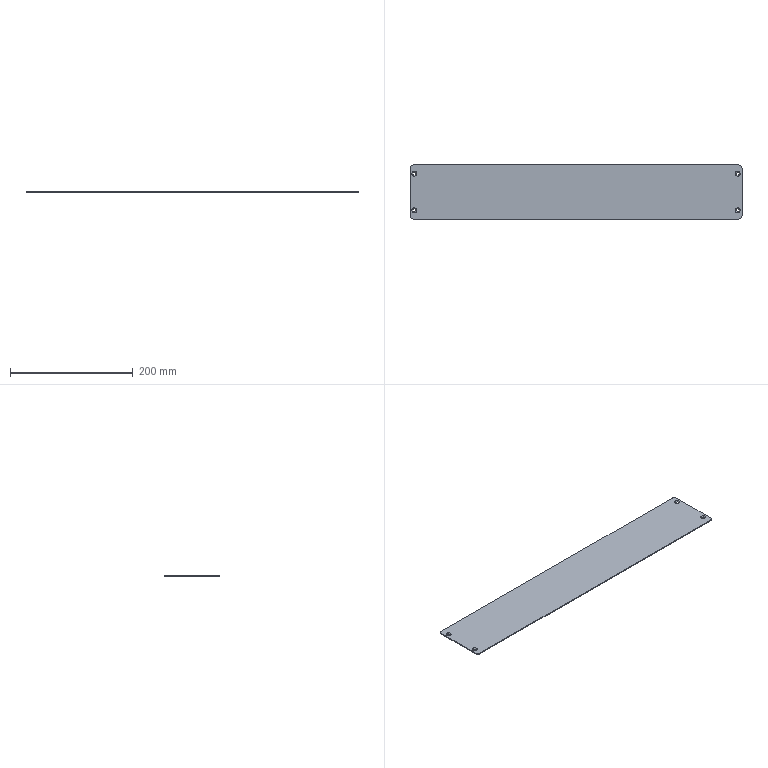Part | SolidWorks | features BreakCorner 1, Chamfer 1, FlatPattern 1, ICE 1, SMBaseFlange 1, SheetMetal 1 | 1 solid | 18 faces | box 541 x 88 x 1.5 mm | volume 71177 mm3 | cone 8 | plane 6 | cylinder 4 | commonest cylinder face diameters 10 x4
STEP:
#1=CARTESIAN_POINT('',(-266.,30.,-1.5));
#2=VERTEX_POINT('',#1);
#3=CARTESIAN_POINT('',(-261.,30.,-1.5));
#4=VERTEX_POINT('',#3);
#5=CARTESIAN_POINT('',(-263.5,30.,-1.5));
#6=DIRECTION('',(0.,0.,1.));
#7=DIRECTION('',(1.,0.,0.));
#8=AXIS2_PLACEMENT_3D('',#5,#6,#7);
#9=CIRCLE('',#8,2.5);
#10=EDGE_CURVE('',#2,#4,#9,.T.);
#11=ORIENTED_EDGE('',*,*,#10,.F.);
#12=CARTESIAN_POINT('',(-267.5,30.,0.));
#13=VERTEX_POINT('',#12);
#14=CARTESIAN_POINT('',(-266.,30.,-1.5));
#15=DIRECTION('',(-0.7071,0.,0.7071));
#16=VECTOR('',#15,1000.);
#17=LINE('',#14,#16);
#18=EDGE_CURVE('',#2,#13,#17,.T.);
#19=ORIENTED_EDGE('',*,*,#18,.T.);
#20=CARTESIAN_POINT('',(-259.5,30.,0.));
#21=VERTEX_POINT('',#20);
#22=CARTESIAN_POINT('',(-263.5,30.,0.));
#23=DIRECTION('',(0.,0.,-1.));
#24=DIRECTION('',(1.,0.,0.));
#25=AXIS2_PLACEMENT_3D('',#22,#23,#24);
#26=CIRCLE('',#25,4.);
#27=EDGE_CURVE('',#21,#13,#26,.T.);
#28=ORIENTED_EDGE('',*,*,#27,.F.);
#29=CARTESIAN_POINT('',(-261.,30.,-1.5));
#30=DIRECTION('',(0.7071,0.,0.7071));
#31=VECTOR('',#30,1000.);
#32=LINE('',#29,#31);
#33=EDGE_CURVE('',#4,#21,#32,.T.);
#34=ORIENTED_EDGE('',*,*,#33,.F.);
#35=EDGE_LOOP('',(#11,#19,#28,#34));
#36=FACE_OUTER_BOUND('',#35,.T.);
#37=CARTESIAN_POINT('',(-263.5,30.,-1.5));
#38=DIRECTION('',(0.,0.,1.));
#39=DIRECTION('',(1.,0.,0.));
#40=AXIS2_PLACEMENT_3D('',#37,#38,#39);
#41=CONICAL_SURFACE('',#40,2.5,0.7854);
#42=ADVANCED_FACE('',(#36),#41,.F.);
#43=CARTESIAN_POINT('',(-266.,-30.,-1.5));
#44=VERTEX_POINT('',#43);
#45=CARTESIAN_POINT('',(-261.,-30.,-1.5));
#46=VERTEX_POINT('',#45);
#47=CARTESIAN_POINT('',(-263.5,-30.,-1.5));
#48=DIRECTION('',(0.,0.,1.));
#49=DIRECTION('',(1.,0.,0.));
#50=AXIS2_PLACEMENT_3D('',#47,#48,#49);
#51=CIRCLE('',#50,2.5);
#52=EDGE_CURVE('',#44,#46,#51,.T.);
#53=ORIENTED_EDGE('',*,*,#52,.F.);
#54=CARTESIAN_POINT('',(-267.5,-30.,0.));
#55=VERTEX_POINT('',#54);
#56=CARTESIAN_POINT('',(-266.,-30.,-1.5));
#57=DIRECTION('',(-0.7071,0.,0.7071));
#58=VECTOR('',#57,1000.);
#59=LINE('',#56,#58);
#60=EDGE_CURVE('',#44,#55,#59,.T.);
#61=ORIENTED_EDGE('',*,*,#60,.T.);
#62=CARTESIAN_POINT('',(-259.5,-30.,0.));
#63=VERTEX_POINT('',#62);
#64=CARTESIAN_POINT('',(-263.5,-30.,0.));
#65=DIRECTION('',(0.,0.,-1.));
#66=DIRECTION('',(1.,0.,0.));
#67=AXIS2_PLACEMENT_3D('',#64,#65,#66);
#68=CIRCLE('',#67,4.);
#69=EDGE_CURVE('',#63,#55,#68,.T.);
#70=ORIENTED_EDGE('',*,*,#69,.F.);
#71=CARTESIAN_POINT('',(-261.,-30.,-1.5));
#72=DIRECTION('',(0.7071,0.,0.7071));
#73=VECTOR('',#72,1000.);
#74=LINE('',#71,#73);
#75=EDGE_CURVE('',#46,#63,#74,.T.);
#76=ORIENTED_EDGE('',*,*,#75,.F.);
#77=EDGE_LOOP('',(#53,#61,#70,#76));
#78=FACE_OUTER_BOUND('',#77,.T.);
#79=CARTESIAN_POINT('',(-263.5,-30.,-1.5));
#80=DIRECTION('',(0.,0.,1.));
#81=DIRECTION('',(1.,0.,0.));
#82=AXIS2_PLACEMENT_3D('',#79,#80,#81);
#83=CONICAL_SURFACE('',#82,2.5,0.7854);
#84=ADVANCED_FACE('',(#78),#83,.F.);
#85=CARTESIAN_POINT('',(261.,30.,-1.5));
#86=VERTEX_POINT('',#85);
#87=CARTESIAN_POINT('',(266.,30.,-1.5));
#88=VERTEX_POINT('',#87);
#89=CARTESIAN_POINT('',(263.5,30.,-1.5));
#90=DIRECTION('',(0.,0.,1.));
#91=DIRECTION('',(1.,0.,0.));
#92=AXIS2_PLACEMENT_3D('',#89,#90,#91);
#93=CIRCLE('',#92,2.5);
#94=EDGE_CURVE('',#86,#88,#93,.T.);
#95=ORIENTED_EDGE('',*,*,#94,.F.);
#96=CARTESIAN_POINT('',(259.5,30.,0.));
#97=VERTEX_POINT('',#96);
#98=CARTESIAN_POINT('',(261.,30.,-1.5));
#99=DIRECTION('',(-0.7071,0.,0.7071));
#100=VECTOR('',#99,1000.);
#101=LINE('',#98,#100);
#102=EDGE_CURVE('',#86,#97,#101,.T.);
#103=ORIENTED_EDGE('',*,*,#102,.T.);
#104=CARTESIAN_POINT('',(267.5,30.,0.));
#105=VERTEX_POINT('',#104);
#106=CARTESIAN_POINT('',(263.5,30.,0.));
#107=DIRECTION('',(0.,0.,-1.));
#108=DIRECTION('',(1.,0.,0.));
#109=AXIS2_PLACEMENT_3D('',#106,#107,#108);
#110=CIRCLE('',#109,4.);
#111=EDGE_CURVE('',#105,#97,#110,.T.);
#112=ORIENTED_EDGE('',*,*,#111,.F.);
#113=CARTESIAN_POINT('',(266.,30.,-1.5));
#114=DIRECTION('',(0.7071,0.,0.7071));
#115=VECTOR('',#114,1000.);
#116=LINE('',#113,#115);
#117=EDGE_CURVE('',#88,#105,#116,.T.);
#118=ORIENTED_EDGE('',*,*,#117,.F.);
#119=EDGE_LOOP('',(#95,#103,#112,#118));
#120=FACE_OUTER_BOUND('',#119,.T.);
#121=CARTESIAN_POINT('',(263.5,30.,-1.5));
#122=DIRECTION('',(0.,0.,1.));
#123=DIRECTION('',(1.,0.,0.));
#124=AXIS2_PLACEMENT_3D('',#121,#122,#123);
#125=CONICAL_SURFACE('',#124,2.5,0.7854);
#126=ADVANCED_FACE('',(#120),#125,.F.);
#127=CARTESIAN_POINT('',(261.,-30.,-1.5));
#128=VERTEX_POINT('',#127);
#129=CARTESIAN_POINT('',(266.,-30.,-1.5));
#130=VERTEX_POINT('',#129);
#131=CARTESIAN_POINT('',(263.5,-30.,-1.5));
#132=DIRECTION('',(0.,0.,1.));
#133=DIRECTION('',(1.,0.,0.));
#134=AXIS2_PLACEMENT_3D('',#131,#132,#133);
#135=CIRCLE('',#134,2.5);
#136=EDGE_CURVE('',#128,#130,#135,.T.);
#137=ORIENTED_EDGE('',*,*,#136,.F.);
#138=CARTESIAN_POINT('',(259.5,-30.,0.));
#139=VERTEX_POINT('',#138);
#140=CARTESIAN_POINT('',(261.,-30.,-1.5));
#141=DIRECTION('',(-0.7071,0.,0.7071));
#142=VECTOR('',#141,1000.);
#143=LINE('',#140,#142);
#144=EDGE_CURVE('',#128,#139,#143,.T.);
#145=ORIENTED_EDGE('',*,*,#144,.T.);
#146=CARTESIAN_POINT('',(267.5,-30.,0.));
#147=VERTEX_POINT('',#146);
#148=CARTESIAN_POINT('',(263.5,-30.,0.));
#149=DIRECTION('',(0.,0.,-1.));
#150=DIRECTION('',(1.,0.,0.));
#151=AXIS2_PLACEMENT_3D('',#148,#149,#150);
#152=CIRCLE('',#151,4.);
#153=EDGE_CURVE('',#147,#139,#152,.T.);
#154=ORIENTED_EDGE('',*,*,#153,.F.);
#155=CARTESIAN_POINT('',(266.,-30.,-1.5));
#156=DIRECTION('',(0.7071,0.,0.7071));
#157=VECTOR('',#156,1000.);
#158=LINE('',#155,#157);
#159=EDGE_CURVE('',#130,#147,#158,.T.);
#160=ORIENTED_EDGE('',*,*,#159,.F.);
#161=EDGE_LOOP('',(#137,#145,#154,#160));
#162=FACE_OUTER_BOUND('',#161,.T.);
#163=CARTESIAN_POINT('',(263.5,-30.,-1.5));
#164=DIRECTION('',(0.,0.,1.));
#165=DIRECTION('',(1.,0.,0.));
#166=AXIS2_PLACEMENT_3D('',#163,#164,#165);
#167=CONICAL_SURFACE('',#166,2.5,0.7854);
#168=ADVANCED_FACE('',(#162),#167,.F.);
#169=CARTESIAN_POINT('',(270.5,-39.,-1.5));
#170=VERTEX_POINT('',#169);
#171=CARTESIAN_POINT('',(270.5,39.,-1.5));
#172=VERTEX_POINT('',#171);
#173=CARTESIAN_POINT('',(270.5,44.,-1.5));
#174=DIRECTION('',(0.,1.,0.));
#175=VECTOR('',#174,1000.);
#176=LINE('',#173,#175);
#177=EDGE_CURVE('',#170,#172,#176,.T.);
#178=ORIENTED_EDGE('',*,*,#177,.T.);
#179=CARTESIAN_POINT('',(270.5,39.,0.));
#180=VERTEX_POINT('',#179);
#181=CARTESIAN_POINT('',(270.5,39.,-1.5));
#182=DIRECTION('',(0.,0.,1.));
#183=VECTOR('',#182,1000.);
#184=LINE('',#181,#183);
#185=EDGE_CURVE('',#172,#180,#184,.T.);
#186=ORIENTED_EDGE('',*,*,#185,.T.);
#187=CARTESIAN_POINT('',(270.5,-39.,0.));
#188=VERTEX_POINT('',#187);
#189=CARTESIAN_POINT('',(270.5,44.,0.));
#190=DIRECTION('',(0.,1.,0.));
#191=VECTOR('',#190,1000.);
#192=LINE('',#189,#191);
#193=EDGE_CURVE('',#188,#180,#192,.T.);
#194=ORIENTED_EDGE('',*,*,#193,.F.);
#195=CARTESIAN_POINT('',(270.5,-39.,-1.5));
#196=DIRECTION('',(0.,0.,-1.));
#197=VECTOR('',#196,1000.);
#198=LINE('',#195,#197);
#199=EDGE_CURVE('',#188,#170,#198,.T.);
#200=ORIENTED_EDGE('',*,*,#199,.T.);
#201=EDGE_LOOP('',(#178,#186,#194,#200));
#202=FACE_OUTER_BOUND('',#201,.T.);
#203=CARTESIAN_POINT('',(270.5,44.,-1.5));
#204=DIRECTION('',(1.,0.,0.));
#205=DIRECTION('',(0.,0.,-1.));
#206=AXIS2_PLACEMENT_3D('',#203,#204,#205);
#207=PLANE('',#206);
#208=ADVANCED_FACE('',(#202),#207,.T.);
#209=CARTESIAN_POINT('',(-265.5,-44.,-1.5));
#210=VERTEX_POINT('',#209);
#211=CARTESIAN_POINT('',(265.5,-44.,-1.5));
#212=VERTEX_POINT('',#211);
#213=CARTESIAN_POINT('',(-270.5,-44.,-1.5));
#214=DIRECTION('',(1.,0.,0.));
#215=VECTOR('',#214,1000.);
#216=LINE('',#213,#215);
#217=EDGE_CURVE('',#210,#212,#216,.T.);
#218=ORIENTED_EDGE('',*,*,#217,.T.);
#219=CARTESIAN_POINT('',(265.5,-44.,0.));
#220=VERTEX_POINT('',#219);
#221=CARTESIAN_POINT('',(265.5,-44.,-1.5));
#222=DIRECTION('',(0.,0.,1.));
#223=VECTOR('',#222,1000.);
#224=LINE('',#221,#223);
#225=EDGE_CURVE('',#212,#220,#224,.T.);
#226=ORIENTED_EDGE('',*,*,#225,.T.);
#227=CARTESIAN_POINT('',(-265.5,-44.,0.));
#228=VERTEX_POINT('',#227);
#229=CARTESIAN_POINT('',(-270.5,-44.,0.));
#230=DIRECTION('',(1.,0.,0.));
#231=VECTOR('',#230,1000.);
#232=LINE('',#229,#231);
#233=EDGE_CURVE('',#228,#220,#232,.T.);
#234=ORIENTED_EDGE('',*,*,#233,.F.);
#235=CARTESIAN_POINT('',(-265.5,-44.,-1.5));
#236=DIRECTION('',(0.,0.,-1.));
#237=VECTOR('',#236,1000.);
#238=LINE('',#235,#237);
#239=EDGE_CURVE('',#228,#210,#238,.T.);
#240=ORIENTED_EDGE('',*,*,#239,.T.);
#241=EDGE_LOOP('',(#218,#226,#234,#240));
#242=FACE_OUTER_BOUND('',#241,.T.);
#243=CARTESIAN_POINT('',(-270.5,-44.,-1.5));
#244=DIRECTION('',(0.,-1.,0.));
#245=DIRECTION('',(0.,0.,-1.));
#246=AXIS2_PLACEMENT_3D('',#243,#244,#245);
#247=PLANE('',#246);
#248=ADVANCED_FACE('',(#242),#247,.T.);
#249=CARTESIAN_POINT('',(-270.5,39.,-1.5));
#250=VERTEX_POINT('',#249);
#251=CARTESIAN_POINT('',(-270.5,-39.,-1.5));
#252=VERTEX_POINT('',#251);
#253=CARTESIAN_POINT('',(-270.5,44.,-1.5));
#254=DIRECTION('',(0.,-1.,0.));
#255=VECTOR('',#254,1000.);
#256=LINE('',#253,#255);
#257=EDGE_CURVE('',#250,#252,#256,.T.);
#258=ORIENTED_EDGE('',*,*,#257,.T.);
#259=CARTESIAN_POINT('',(-270.5,-39.,0.));
#260=VERTEX_POINT('',#259);
#261=CARTESIAN_POINT('',(-270.5,-39.,-1.5));
#262=DIRECTION('',(0.,0.,1.));
#263=VECTOR('',#262,1000.);
#264=LINE('',#261,#263);
#265=EDGE_CURVE('',#252,#260,#264,.T.);
#266=ORIENTED_EDGE('',*,*,#265,.T.);
#267=CARTESIAN_POINT('',(-270.5,39.,0.));
#268=VERTEX_POINT('',#267);
#269=CARTESIAN_POINT('',(-270.5,44.,0.));
#270=DIRECTION('',(0.,-1.,0.));
#271=VECTOR('',#270,1000.);
#272=LINE('',#269,#271);
#273=EDGE_CURVE('',#268,#260,#272,.T.);
#274=ORIENTED_EDGE('',*,*,#273,.F.);
#275=CARTESIAN_POINT('',(-270.5,39.,-1.5));
#276=DIRECTION('',(0.,0.,-1.));
#277=VECTOR('',#276,1000.);
#278=LINE('',#275,#277);
#279=EDGE_CURVE('',#268,#250,#278,.T.);
#280=ORIENTED_EDGE('',*,*,#279,.T.);
#281=EDGE_LOOP('',(#258,#266,#274,#280));
#282=FACE_OUTER_BOUND('',#281,.T.);
#283=CARTESIAN_POINT('',(-270.5,44.,-1.5));
#284=DIRECTION('',(-1.,0.,0.));
#285=DIRECTION('',(0.,0.,1.));
#286=AXIS2_PLACEMENT_3D('',#283,#284,#285);
#287=PLANE('',#286);
#288=ADVANCED_FACE('',(#282),#287,.T.);
#289=CARTESIAN_POINT('',(265.5,44.,0.));
#290=VERTEX_POINT('',#289);
#291=CARTESIAN_POINT('',(-265.5,44.,0.));
#292=VERTEX_POINT('',#291);
#293=CARTESIAN_POINT('',(-270.5,44.,0.));
#294=DIRECTION('',(-1.,0.,0.));
#295=VECTOR('',#294,1000.);
#296=LINE('',#293,#295);
#297=EDGE_CURVE('',#290,#292,#296,.T.);
#298=ORIENTED_EDGE('',*,*,#297,.F.);
#299=CARTESIAN_POINT('',(265.5,44.,-1.5));
#300=VERTEX_POINT('',#299);
#301=CARTESIAN_POINT('',(265.5,44.,-1.5));
#302=DIRECTION('',(0.,0.,-1.));
#303=VECTOR('',#302,1000.);
#304=LINE('',#301,#303);
#305=EDGE_CURVE('',#290,#300,#304,.T.);
#306=ORIENTED_EDGE('',*,*,#305,.T.);
#307=CARTESIAN_POINT('',(-265.5,44.,-1.5));
#308=VERTEX_POINT('',#307);
#309=CARTESIAN_POINT('',(-270.5,44.,-1.5));
#310=DIRECTION('',(-1.,0.,0.));
#311=VECTOR('',#310,1000.);
#312=LINE('',#309,#311);
#313=EDGE_CURVE('',#300,#308,#312,.T.);
#314=ORIENTED_EDGE('',*,*,#313,.T.);
#315=CARTESIAN_POINT('',(-265.5,44.,-1.5));
#316=DIRECTION('',(0.,0.,1.));
#317=VECTOR('',#316,1000.);
#318=LINE('',#315,#317);
#319=EDGE_CURVE('',#308,#292,#318,.T.);
#320=ORIENTED_EDGE('',*,*,#319,.T.);
#321=EDGE_LOOP('',(#298,#306,#314,#320));
#322=FACE_OUTER_BOUND('',#321,.T.);
#323=CARTESIAN_POINT('',(-270.5,44.,-1.5));
#324=DIRECTION('',(0.,1.,0.));
#325=DIRECTION('',(0.,0.,1.));
#326=AXIS2_PLACEMENT_3D('',#323,#324,#325);
#327=PLANE('',#326);
#328=ADVANCED_FACE('',(#322),#327,.T.);
#329=CARTESIAN_POINT('',(-263.5,-30.,-1.5));
#330=DIRECTION('',(0.,0.,1.));
#331=DIRECTION('',(1.,0.,0.));
#332=AXIS2_PLACEMENT_3D('',#329,#330,#331);
#333=CIRCLE('',#332,2.5);
#334=EDGE_CURVE('',#46,#44,#333,.T.);
#335=ORIENTED_EDGE('',*,*,#334,.T.);
#336=ORIENTED_EDGE('',*,*,#52,.T.);
#337=EDGE_LOOP('',(#335,#336));
#338=FACE_BOUND('',#337,.T.);
#339=CARTESIAN_POINT('',(263.5,-30.,-1.5));
#340=DIRECTION('',(0.,0.,1.));
#341=DIRECTION('',(1.,0.,0.));
#342=AXIS2_PLACEMENT_3D('',#339,#340,#341);
#343=CIRCLE('',#342,2.5);
#344=EDGE_CURVE('',#130,#128,#343,.T.);
#345=ORIENTED_EDGE('',*,*,#344,.T.);
#346=ORIENTED_EDGE('',*,*,#136,.T.);
#347=EDGE_LOOP('',(#345,#346));
#348=FACE_BOUND('',#347,.T.);
#349=CARTESIAN_POINT('',(263.5,30.,-1.5));
#350=DIRECTION('',(0.,0.,1.));
#351=DIRECTION('',(1.,0.,0.));
#352=AXIS2_PLACEMENT_3D('',#349,#350,#351);
#353=CIRCLE('',#352,2.5);
#354=EDGE_CURVE('',#88,#86,#353,.T.);
#355=ORIENTED_EDGE('',*,*,#354,.T.);
#356=ORIENTED_EDGE('',*,*,#94,.T.);
#357=EDGE_LOOP('',(#355,#356));
#358=FACE_BOUND('',#357,.T.);
#359=CARTESIAN_POINT('',(-263.5,30.,-1.5));
#360=DIRECTION('',(0.,0.,1.));
#361=DIRECTION('',(1.,0.,0.));
#362=AXIS2_PLACEMENT_3D('',#359,#360,#361);
#363=CIRCLE('',#362,2.5);
#364=EDGE_CURVE('',#4,#2,#363,.T.);
#365=ORIENTED_EDGE('',*,*,#364,.T.);
#366=ORIENTED_EDGE('',*,*,#10,.T.);
#367=EDGE_LOOP('',(#365,#366));
#368=FACE_BOUND('',#367,.T.);
#369=ORIENTED_EDGE('',*,*,#313,.F.);
#370=CARTESIAN_POINT('',(265.5,39.,-1.5));
#371=DIRECTION('',(0.,0.,-1.));
#372=DIRECTION('',(1.,0.,0.));
#373=AXIS2_PLACEMENT_3D('',#370,#371,#372);
#374=CIRCLE('',#373,5.);
#375=EDGE_CURVE('',#300,#172,#374,.T.);
#376=ORIENTED_EDGE('',*,*,#375,.T.);
#377=ORIENTED_EDGE('',*,*,#177,.F.);
#378=CARTESIAN_POINT('',(265.5,-39.,-1.5));
#379=DIRECTION('',(0.,0.,-1.));
#380=DIRECTION('',(1.,0.,0.));
#381=AXIS2_PLACEMENT_3D('',#378,#379,#380);
#382=CIRCLE('',#381,5.);
#383=EDGE_CURVE('',#170,#212,#382,.T.);
#384=ORIENTED_EDGE('',*,*,#383,.T.);
#385=ORIENTED_EDGE('',*,*,#217,.F.);
#386=CARTESIAN_POINT('',(-265.5,-39.,-1.5));
#387=DIRECTION('',(0.,0.,-1.));
#388=DIRECTION('',(1.,0.,0.));
#389=AXIS2_PLACEMENT_3D('',#386,#387,#388);
#390=CIRCLE('',#389,5.);
#391=EDGE_CURVE('',#210,#252,#390,.T.);
#392=ORIENTED_EDGE('',*,*,#391,.T.);
#393=ORIENTED_EDGE('',*,*,#257,.F.);
#394=CARTESIAN_POINT('',(-265.5,39.,-1.5));
#395=DIRECTION('',(0.,0.,-1.));
#396=DIRECTION('',(1.,0.,0.));
#397=AXIS2_PLACEMENT_3D('',#394,#395,#396);
#398=CIRCLE('',#397,5.);
#399=EDGE_CURVE('',#250,#308,#398,.T.);
#400=ORIENTED_EDGE('',*,*,#399,.T.);
#401=EDGE_LOOP('',(#369,#376,#377,#384,#385,#392,#393,#400));
#402=FACE_OUTER_BOUND('',#401,.T.);
#403=CARTESIAN_POINT('',(0.,0.,-1.5));
#404=DIRECTION('',(0.,0.,1.));
#405=DIRECTION('',(1.,0.,0.));
#406=AXIS2_PLACEMENT_3D('',#403,#404,#405);
#407=PLANE('',#406);
#408=ADVANCED_FACE('',(#338,#348,#358,#368,#402),#407,.F.);
#409=ORIENTED_EDGE('',*,*,#153,.T.);
#410=CARTESIAN_POINT('',(263.5,-30.,0.));
#411=DIRECTION('',(0.,0.,-1.));
#412=DIRECTION('',(1.,0.,0.));
#413=AXIS2_PLACEMENT_3D('',#410,#411,#412);
#414=CIRCLE('',#413,4.);
#415=EDGE_CURVE('',#139,#147,#414,.T.);
#416=ORIENTED_EDGE('',*,*,#415,.T.);
#417=EDGE_LOOP('',(#409,#416));
#418=FACE_BOUND('',#417,.T.);
#419=ORIENTED_EDGE('',*,*,#111,.T.);
#420=CARTESIAN_POINT('',(263.5,30.,0.));
#421=DIRECTION('',(0.,0.,-1.));
#422=DIRECTION('',(1.,0.,0.));
#423=AXIS2_PLACEMENT_3D('',#420,#421,#422);
#424=CIRCLE('',#423,4.);
#425=EDGE_CURVE('',#97,#105,#424,.T.);
#426=ORIENTED_EDGE('',*,*,#425,.T.);
#427=EDGE_LOOP('',(#419,#426));
#428=FACE_BOUND('',#427,.T.);
#429=ORIENTED_EDGE('',*,*,#69,.T.);
#430=CARTESIAN_POINT('',(-263.5,-30.,0.));
#431=DIRECTION('',(0.,0.,-1.));
#432=DIRECTION('',(1.,0.,0.));
#433=AXIS2_PLACEMENT_3D('',#430,#431,#432);
#434=CIRCLE('',#433,4.);
#435=EDGE_CURVE('',#55,#63,#434,.T.);
#436=ORIENTED_EDGE('',*,*,#435,.T.);
#437=EDGE_LOOP('',(#429,#436));
#438=FACE_BOUND('',#437,.T.);
#439=ORIENTED_EDGE('',*,*,#27,.T.);
#440=CARTESIAN_POINT('',(-263.5,30.,0.));
#441=DIRECTION('',(0.,0.,-1.));
#442=DIRECTION('',(1.,0.,0.));
#443=AXIS2_PLACEMENT_3D('',#440,#441,#442);
#444=CIRCLE('',#443,4.);
#445=EDGE_CURVE('',#13,#21,#444,.T.);
#446=ORIENTED_EDGE('',*,*,#445,.T.);
#447=EDGE_LOOP('',(#439,#446));
#448=FACE_BOUND('',#447,.T.);
#449=ORIENTED_EDGE('',*,*,#193,.T.);
#450=CARTESIAN_POINT('',(265.5,39.,0.));
#451=DIRECTION('',(0.,0.,1.));
#452=DIRECTION('',(1.,0.,0.));
#453=AXIS2_PLACEMENT_3D('',#450,#451,#452);
#454=CIRCLE('',#453,5.);
#455=EDGE_CURVE('',#180,#290,#454,.T.);
#456=ORIENTED_EDGE('',*,*,#455,.T.);
#457=ORIENTED_EDGE('',*,*,#297,.T.);
#458=CARTESIAN_POINT('',(-265.5,39.,0.));
#459=DIRECTION('',(0.,0.,1.));
#460=DIRECTION('',(1.,0.,0.));
#461=AXIS2_PLACEMENT_3D('',#458,#459,#460);
#462=CIRCLE('',#461,5.);
#463=EDGE_CURVE('',#292,#268,#462,.T.);
#464=ORIENTED_EDGE('',*,*,#463,.T.);
#465=ORIENTED_EDGE('',*,*,#273,.T.);
#466=CARTESIAN_POINT('',(-265.5,-39.,0.));
#467=DIRECTION('',(0.,0.,1.));
#468=DIRECTION('',(1.,0.,0.));
#469=AXIS2_PLACEMENT_3D('',#466,#467,#468);
#470=CIRCLE('',#469,5.);
#471=EDGE_CURVE('',#260,#228,#470,.T.);
#472=ORIENTED_EDGE('',*,*,#471,.T.);
#473=ORIENTED_EDGE('',*,*,#233,.T.);
#474=CARTESIAN_POINT('',(265.5,-39.,0.));
#475=DIRECTION('',(0.,0.,1.));
#476=DIRECTION('',(1.,0.,0.));
#477=AXIS2_PLACEMENT_3D('',#474,#475,#476);
#478=CIRCLE('',#477,5.);
#479=EDGE_CURVE('',#220,#188,#478,.T.);
#480=ORIENTED_EDGE('',*,*,#479,.T.);
#481=EDGE_LOOP('',(#449,#456,#457,#464,#465,#472,#473,#480));
#482=FACE_OUTER_BOUND('',#481,.T.);
#483=CARTESIAN_POINT('',(0.,0.,0.));
#484=DIRECTION('',(0.,0.,1.));
#485=DIRECTION('',(1.,0.,0.));
#486=AXIS2_PLACEMENT_3D('',#483,#484,#485);
#487=PLANE('',#486);
#488=ADVANCED_FACE('',(#418,#428,#438,#448,#482),#487,.T.);
#489=ORIENTED_EDGE('',*,*,#144,.F.);
#490=ORIENTED_EDGE('',*,*,#344,.F.);
#491=ORIENTED_EDGE('',*,*,#159,.T.);
#492=ORIENTED_EDGE('',*,*,#415,.F.);
#493=EDGE_LOOP('',(#489,#490,#491,#492));
#494=FACE_OUTER_BOUND('',#493,.T.);
#495=CARTESIAN_POINT('',(263.5,-30.,-1.5));
#496=DIRECTION('',(0.,0.,1.));
#497=DIRECTION('',(1.,0.,0.));
#498=AXIS2_PLACEMENT_3D('',#495,#496,#497);
#499=CONICAL_SURFACE('',#498,2.5,0.7854);
#500=ADVANCED_FACE('',(#494),#499,.F.);
#501=ORIENTED_EDGE('',*,*,#102,.F.);
#502=ORIENTED_EDGE('',*,*,#354,.F.);
#503=ORIENTED_EDGE('',*,*,#117,.T.);
#504=ORIENTED_EDGE('',*,*,#425,.F.);
#505=EDGE_LOOP('',(#501,#502,#503,#504));
#506=FACE_OUTER_BOUND('',#505,.T.);
#507=CARTESIAN_POINT('',(263.5,30.,-1.5));
#508=DIRECTION('',(0.,0.,1.));
#509=DIRECTION('',(1.,0.,0.));
#510=AXIS2_PLACEMENT_3D('',#507,#508,#509);
#511=CONICAL_SURFACE('',#510,2.5,0.7854);
#512=ADVANCED_FACE('',(#506),#511,.F.);
#513=ORIENTED_EDGE('',*,*,#60,.F.);
#514=ORIENTED_EDGE('',*,*,#334,.F.);
#515=ORIENTED_EDGE('',*,*,#75,.T.);
#516=ORIENTED_EDGE('',*,*,#435,.F.);
#517=EDGE_LOOP('',(#513,#514,#515,#516));
#518=FACE_OUTER_BOUND('',#517,.T.);
#519=CARTESIAN_POINT('',(-263.5,-30.,-1.5));
#520=DIRECTION('',(0.,0.,1.));
#521=DIRECTION('',(1.,0.,0.));
#522=AXIS2_PLACEMENT_3D('',#519,#520,#521);
#523=CONICAL_SURFACE('',#522,2.5,0.7854);
#524=ADVANCED_FACE('',(#518),#523,.F.);
#525=ORIENTED_EDGE('',*,*,#18,.F.);
#526=ORIENTED_EDGE('',*,*,#364,.F.);
#527=ORIENTED_EDGE('',*,*,#33,.T.);
#528=ORIENTED_EDGE('',*,*,#445,.F.);
#529=EDGE_LOOP('',(#525,#526,#527,#528));
#530=FACE_OUTER_BOUND('',#529,.T.);
#531=CARTESIAN_POINT('',(-263.5,30.,-1.5));
#532=DIRECTION('',(0.,0.,1.));
#533=DIRECTION('',(1.,0.,0.));
#534=AXIS2_PLACEMENT_3D('',#531,#532,#533);
#535=CONICAL_SURFACE('',#534,2.5,0.7854);
#536=ADVANCED_FACE('',(#530),#535,.F.);
#537=ORIENTED_EDGE('',*,*,#375,.F.);
#538=ORIENTED_EDGE('',*,*,#305,.F.);
#539=ORIENTED_EDGE('',*,*,#455,.F.);
#540=ORIENTED_EDGE('',*,*,#185,.F.);
#541=EDGE_LOOP('',(#537,#538,#539,#540));
#542=FACE_OUTER_BOUND('',#541,.T.);
#543=CARTESIAN_POINT('',(265.5,39.,-1.5));
#544=DIRECTION('',(0.,0.,1.));
#545=DIRECTION('',(1.,0.,0.));
#546=AXIS2_PLACEMENT_3D('',#543,#544,#545);
#547=CYLINDRICAL_SURFACE('',#546,5.);
#548=ADVANCED_FACE('',(#542),#547,.T.);
#549=ORIENTED_EDGE('',*,*,#383,.F.);
#550=ORIENTED_EDGE('',*,*,#199,.F.);
#551=ORIENTED_EDGE('',*,*,#479,.F.);
#552=ORIENTED_EDGE('',*,*,#225,.F.);
#553=EDGE_LOOP('',(#549,#550,#551,#552));
#554=FACE_OUTER_BOUND('',#553,.T.);
#555=CARTESIAN_POINT('',(265.5,-39.,-1.5));
#556=DIRECTION('',(0.,0.,1.));
#557=DIRECTION('',(1.,0.,0.));
#558=AXIS2_PLACEMENT_3D('',#555,#556,#557);
#559=CYLINDRICAL_SURFACE('',#558,5.);
#560=ADVANCED_FACE('',(#554),#559,.T.);
#561=ORIENTED_EDGE('',*,*,#391,.F.);
#562=ORIENTED_EDGE('',*,*,#239,.F.);
#563=ORIENTED_EDGE('',*,*,#471,.F.);
#564=ORIENTED_EDGE('',*,*,#265,.F.);
#565=EDGE_LOOP('',(#561,#562,#563,#564));
#566=FACE_OUTER_BOUND('',#565,.T.);
#567=CARTESIAN_POINT('',(-265.5,-39.,-1.5));
#568=DIRECTION('',(0.,0.,1.));
#569=DIRECTION('',(1.,0.,0.));
#570=AXIS2_PLACEMENT_3D('',#567,#568,#569);
#571=CYLINDRICAL_SURFACE('',#570,5.);
#572=ADVANCED_FACE('',(#566),#571,.T.);
#573=ORIENTED_EDGE('',*,*,#399,.F.);
#574=ORIENTED_EDGE('',*,*,#279,.F.);
#575=ORIENTED_EDGE('',*,*,#463,.F.);
#576=ORIENTED_EDGE('',*,*,#319,.F.);
#577=EDGE_LOOP('',(#573,#574,#575,#576));
#578=FACE_OUTER_BOUND('',#577,.T.);
#579=CARTESIAN_POINT('',(-265.5,39.,-1.5));
#580=DIRECTION('',(0.,0.,1.));
#581=DIRECTION('',(1.,0.,0.));
#582=AXIS2_PLACEMENT_3D('',#579,#580,#581);
#583=CYLINDRICAL_SURFACE('',#582,5.);
#584=ADVANCED_FACE('',(#578),#583,.T.);
#585=CLOSED_SHELL('',(#42,#84,#126,#168,#208,#248,#288,#328,#408,#488,#500,#512,#524,#536,#548,#560,#572,#584));
#586=MANIFOLD_SOLID_BREP('',#585);
#587=CARTESIAN_POINT('',(0.,0.,0.));
#588=DIRECTION('',(0.,0.,1.));
#589=DIRECTION('',(1.,0.,0.));
#590=AXIS2_PLACEMENT_3D('',#587,#588,#589);
#591=(LENGTH_UNIT()NAMED_UNIT(*)SI_UNIT(.MILLI.,.METRE.));
#592=UNCERTAINTY_MEASURE_WITH_UNIT(LENGTH_MEASURE(0.00001),#591,'','');
#593=(NAMED_UNIT(*)PLANE_ANGLE_UNIT()SI_UNIT($,.RADIAN.));
#594=(NAMED_UNIT(*)SI_UNIT($,.STERADIAN.)SOLID_ANGLE_UNIT());
#595=(GEOMETRIC_REPRESENTATION_CONTEXT(3)GLOBAL_UNCERTAINTY_ASSIGNED_CONTEXT((#592))GLOBAL_UNIT_ASSIGNED_CONTEXT((#591,#593,#594))REPRESENTATION_CONTEXT('',''));
#596=ADVANCED_BREP_SHAPE_REPRESENTATION('',(#586,#590),#595);